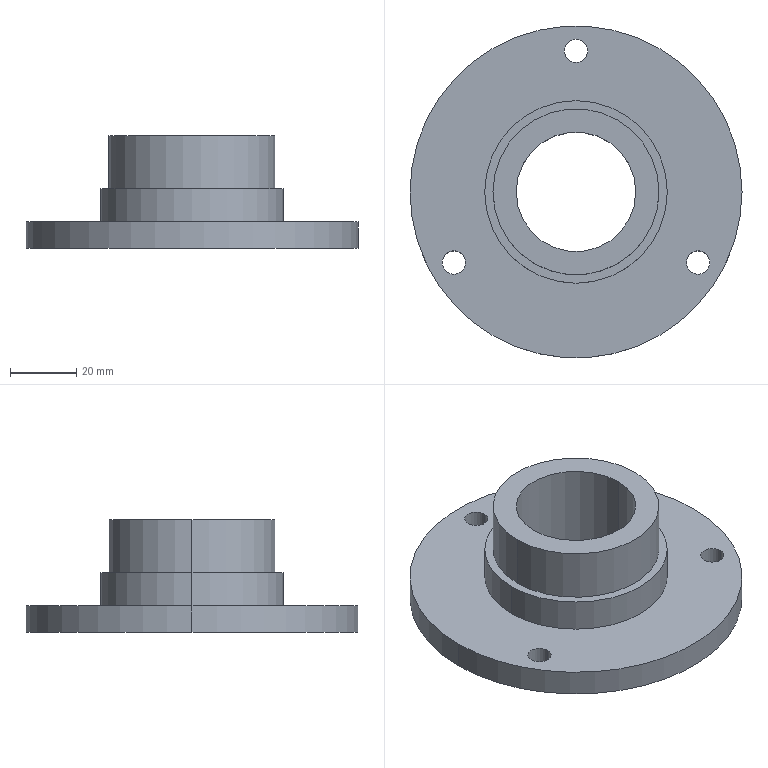Part | SolidWorks | features ICE 2, Extrusion 1 | 1 solid | 18 faces | box 100 x 100 x 34 mm | volume 82475 mm3 | cylinder 14 | plane 4 | commonest cylinder face diameters 7 x6 36 x2 50 x2 55 x2 100 x2
STEP:
#1=CARTESIAN_POINT('',(25.,0.,34.));
#2=VERTEX_POINT('',#1);
#3=CARTESIAN_POINT('',(-25.,0.,34.));
#4=VERTEX_POINT('',#3);
#5=CARTESIAN_POINT('',(0.,0.,34.));
#6=DIRECTION('',(0.,0.,1.));
#7=DIRECTION('',(1.,0.,0.));
#8=AXIS2_PLACEMENT_3D('',#5,#6,#7);
#9=CIRCLE('',#8,25.);
#10=EDGE_CURVE('',#2,#4,#9,.T.);
#11=ORIENTED_EDGE('',*,*,#10,.F.);
#12=CARTESIAN_POINT('',(25.,0.,18.));
#13=VERTEX_POINT('',#12);
#14=CARTESIAN_POINT('',(25.,0.,34.));
#15=DIRECTION('',(0.,0.,-1.));
#16=VECTOR('',#15,1000.);
#17=LINE('',#14,#16);
#18=EDGE_CURVE('',#2,#13,#17,.T.);
#19=ORIENTED_EDGE('',*,*,#18,.T.);
#20=CARTESIAN_POINT('',(-25.,0.,18.));
#21=VERTEX_POINT('',#20);
#22=CARTESIAN_POINT('',(0.,0.,18.));
#23=DIRECTION('',(0.,0.,1.));
#24=DIRECTION('',(1.,0.,0.));
#25=AXIS2_PLACEMENT_3D('',#22,#23,#24);
#26=CIRCLE('',#25,25.);
#27=EDGE_CURVE('',#13,#21,#26,.T.);
#28=ORIENTED_EDGE('',*,*,#27,.T.);
#29=CARTESIAN_POINT('',(-25.,0.,34.));
#30=DIRECTION('',(0.,0.,-1.));
#31=VECTOR('',#30,1000.);
#32=LINE('',#29,#31);
#33=EDGE_CURVE('',#4,#21,#32,.T.);
#34=ORIENTED_EDGE('',*,*,#33,.F.);
#35=EDGE_LOOP('',(#11,#19,#28,#34));
#36=FACE_OUTER_BOUND('',#35,.T.);
#37=CARTESIAN_POINT('',(0.,0.,34.));
#38=DIRECTION('',(0.,0.,-1.));
#39=DIRECTION('',(-1.,0.,0.));
#40=AXIS2_PLACEMENT_3D('',#37,#38,#39);
#41=CYLINDRICAL_SURFACE('',#40,25.);
#42=ADVANCED_FACE('',(#36),#41,.T.);
#43=CARTESIAN_POINT('',(27.5,0.,18.));
#44=VERTEX_POINT('',#43);
#45=CARTESIAN_POINT('',(-27.5,0.,18.));
#46=VERTEX_POINT('',#45);
#47=CARTESIAN_POINT('',(0.,0.,18.));
#48=DIRECTION('',(0.,0.,1.));
#49=DIRECTION('',(1.,0.,0.));
#50=AXIS2_PLACEMENT_3D('',#47,#48,#49);
#51=CIRCLE('',#50,27.5);
#52=EDGE_CURVE('',#44,#46,#51,.T.);
#53=ORIENTED_EDGE('',*,*,#52,.F.);
#54=CARTESIAN_POINT('',(27.5,0.,8.));
#55=VERTEX_POINT('',#54);
#56=CARTESIAN_POINT('',(27.5,0.,18.));
#57=DIRECTION('',(0.,0.,-1.));
#58=VECTOR('',#57,1000.);
#59=LINE('',#56,#58);
#60=EDGE_CURVE('',#44,#55,#59,.T.);
#61=ORIENTED_EDGE('',*,*,#60,.T.);
#62=CARTESIAN_POINT('',(-27.5,0.,8.));
#63=VERTEX_POINT('',#62);
#64=CARTESIAN_POINT('',(0.,0.,8.));
#65=DIRECTION('',(0.,0.,1.));
#66=DIRECTION('',(1.,0.,0.));
#67=AXIS2_PLACEMENT_3D('',#64,#65,#66);
#68=CIRCLE('',#67,27.5);
#69=EDGE_CURVE('',#55,#63,#68,.T.);
#70=ORIENTED_EDGE('',*,*,#69,.T.);
#71=CARTESIAN_POINT('',(-27.5,0.,18.));
#72=DIRECTION('',(0.,0.,-1.));
#73=VECTOR('',#72,1000.);
#74=LINE('',#71,#73);
#75=EDGE_CURVE('',#46,#63,#74,.T.);
#76=ORIENTED_EDGE('',*,*,#75,.F.);
#77=EDGE_LOOP('',(#53,#61,#70,#76));
#78=FACE_OUTER_BOUND('',#77,.T.);
#79=CARTESIAN_POINT('',(0.,0.,18.));
#80=DIRECTION('',(0.,0.,-1.));
#81=DIRECTION('',(-1.,0.,0.));
#82=AXIS2_PLACEMENT_3D('',#79,#80,#81);
#83=CYLINDRICAL_SURFACE('',#82,27.5);
#84=ADVANCED_FACE('',(#78),#83,.T.);
#85=CARTESIAN_POINT('',(-18.,0.,34.));
#86=VERTEX_POINT('',#85);
#87=CARTESIAN_POINT('',(18.,0.,34.));
#88=VERTEX_POINT('',#87);
#89=CARTESIAN_POINT('',(0.,0.,34.));
#90=DIRECTION('',(0.,0.,1.));
#91=DIRECTION('',(1.,0.,0.));
#92=AXIS2_PLACEMENT_3D('',#89,#90,#91);
#93=CIRCLE('',#92,18.);
#94=EDGE_CURVE('',#86,#88,#93,.T.);
#95=ORIENTED_EDGE('',*,*,#94,.T.);
#96=CARTESIAN_POINT('',(18.,0.,0.));
#97=VERTEX_POINT('',#96);
#98=CARTESIAN_POINT('',(18.,0.,8.));
#99=DIRECTION('',(0.,0.,-1.));
#100=VECTOR('',#99,1000.);
#101=LINE('',#98,#100);
#102=EDGE_CURVE('',#88,#97,#101,.T.);
#103=ORIENTED_EDGE('',*,*,#102,.T.);
#104=CARTESIAN_POINT('',(-18.,0.,0.));
#105=VERTEX_POINT('',#104);
#106=CARTESIAN_POINT('',(0.,0.,0.));
#107=DIRECTION('',(0.,0.,1.));
#108=DIRECTION('',(1.,0.,0.));
#109=AXIS2_PLACEMENT_3D('',#106,#107,#108);
#110=CIRCLE('',#109,18.);
#111=EDGE_CURVE('',#105,#97,#110,.T.);
#112=ORIENTED_EDGE('',*,*,#111,.F.);
#113=CARTESIAN_POINT('',(-18.,0.,8.));
#114=DIRECTION('',(0.,0.,-1.));
#115=VECTOR('',#114,1000.);
#116=LINE('',#113,#115);
#117=EDGE_CURVE('',#86,#105,#116,.T.);
#118=ORIENTED_EDGE('',*,*,#117,.F.);
#119=EDGE_LOOP('',(#95,#103,#112,#118));
#120=FACE_OUTER_BOUND('',#119,.T.);
#121=CARTESIAN_POINT('',(0.,0.,8.));
#122=DIRECTION('',(0.,0.,-1.));
#123=DIRECTION('',(-1.,0.,0.));
#124=AXIS2_PLACEMENT_3D('',#121,#122,#123);
#125=CYLINDRICAL_SURFACE('',#124,18.);
#126=ADVANCED_FACE('',(#120),#125,.F.);
#127=CARTESIAN_POINT('',(33.306,-21.25,8.));
#128=VERTEX_POINT('',#127);
#129=CARTESIAN_POINT('',(40.306,-21.25,8.));
#130=VERTEX_POINT('',#129);
#131=CARTESIAN_POINT('',(36.806,-21.25,8.));
#132=DIRECTION('',(0.,0.,1.));
#133=DIRECTION('',(1.,0.,0.));
#134=AXIS2_PLACEMENT_3D('',#131,#132,#133);
#135=CIRCLE('',#134,3.5);
#136=EDGE_CURVE('',#128,#130,#135,.T.);
#137=ORIENTED_EDGE('',*,*,#136,.T.);
#138=CARTESIAN_POINT('',(40.306,-21.25,0.));
#139=VERTEX_POINT('',#138);
#140=CARTESIAN_POINT('',(40.306,-21.25,8.));
#141=DIRECTION('',(0.,0.,-1.));
#142=VECTOR('',#141,1000.);
#143=LINE('',#140,#142);
#144=EDGE_CURVE('',#130,#139,#143,.T.);
#145=ORIENTED_EDGE('',*,*,#144,.T.);
#146=CARTESIAN_POINT('',(33.306,-21.25,0.));
#147=VERTEX_POINT('',#146);
#148=CARTESIAN_POINT('',(36.806,-21.25,0.));
#149=DIRECTION('',(0.,0.,1.));
#150=DIRECTION('',(1.,0.,0.));
#151=AXIS2_PLACEMENT_3D('',#148,#149,#150);
#152=CIRCLE('',#151,3.5);
#153=EDGE_CURVE('',#147,#139,#152,.T.);
#154=ORIENTED_EDGE('',*,*,#153,.F.);
#155=CARTESIAN_POINT('',(33.306,-21.25,8.));
#156=DIRECTION('',(0.,0.,-1.));
#157=VECTOR('',#156,1000.);
#158=LINE('',#155,#157);
#159=EDGE_CURVE('',#128,#147,#158,.T.);
#160=ORIENTED_EDGE('',*,*,#159,.F.);
#161=EDGE_LOOP('',(#137,#145,#154,#160));
#162=FACE_OUTER_BOUND('',#161,.T.);
#163=CARTESIAN_POINT('',(36.806,-21.25,8.));
#164=DIRECTION('',(0.,0.,-1.));
#165=DIRECTION('',(-1.,0.,0.));
#166=AXIS2_PLACEMENT_3D('',#163,#164,#165);
#167=CYLINDRICAL_SURFACE('',#166,3.5);
#168=ADVANCED_FACE('',(#162),#167,.F.);
#169=CARTESIAN_POINT('',(-40.306,-21.25,8.));
#170=VERTEX_POINT('',#169);
#171=CARTESIAN_POINT('',(-33.306,-21.25,8.));
#172=VERTEX_POINT('',#171);
#173=CARTESIAN_POINT('',(-36.806,-21.25,8.));
#174=DIRECTION('',(0.,0.,1.));
#175=DIRECTION('',(1.,0.,0.));
#176=AXIS2_PLACEMENT_3D('',#173,#174,#175);
#177=CIRCLE('',#176,3.5);
#178=EDGE_CURVE('',#170,#172,#177,.T.);
#179=ORIENTED_EDGE('',*,*,#178,.T.);
#180=CARTESIAN_POINT('',(-33.306,-21.25,0.));
#181=VERTEX_POINT('',#180);
#182=CARTESIAN_POINT('',(-33.306,-21.25,8.));
#183=DIRECTION('',(0.,0.,-1.));
#184=VECTOR('',#183,1000.);
#185=LINE('',#182,#184);
#186=EDGE_CURVE('',#172,#181,#185,.T.);
#187=ORIENTED_EDGE('',*,*,#186,.T.);
#188=CARTESIAN_POINT('',(-40.306,-21.25,0.));
#189=VERTEX_POINT('',#188);
#190=CARTESIAN_POINT('',(-36.806,-21.25,0.));
#191=DIRECTION('',(0.,0.,1.));
#192=DIRECTION('',(1.,0.,0.));
#193=AXIS2_PLACEMENT_3D('',#190,#191,#192);
#194=CIRCLE('',#193,3.5);
#195=EDGE_CURVE('',#189,#181,#194,.T.);
#196=ORIENTED_EDGE('',*,*,#195,.F.);
#197=CARTESIAN_POINT('',(-40.306,-21.25,8.));
#198=DIRECTION('',(0.,0.,-1.));
#199=VECTOR('',#198,1000.);
#200=LINE('',#197,#199);
#201=EDGE_CURVE('',#170,#189,#200,.T.);
#202=ORIENTED_EDGE('',*,*,#201,.F.);
#203=EDGE_LOOP('',(#179,#187,#196,#202));
#204=FACE_OUTER_BOUND('',#203,.T.);
#205=CARTESIAN_POINT('',(-36.806,-21.25,8.));
#206=DIRECTION('',(0.,0.,-1.));
#207=DIRECTION('',(-1.,0.,0.));
#208=AXIS2_PLACEMENT_3D('',#205,#206,#207);
#209=CYLINDRICAL_SURFACE('',#208,3.5);
#210=ADVANCED_FACE('',(#204),#209,.F.);
#211=CARTESIAN_POINT('',(-3.5,42.5,8.));
#212=VERTEX_POINT('',#211);
#213=CARTESIAN_POINT('',(3.5,42.5,8.));
#214=VERTEX_POINT('',#213);
#215=CARTESIAN_POINT('',(0.,42.5,8.));
#216=DIRECTION('',(0.,0.,1.));
#217=DIRECTION('',(1.,0.,0.));
#218=AXIS2_PLACEMENT_3D('',#215,#216,#217);
#219=CIRCLE('',#218,3.5);
#220=EDGE_CURVE('',#212,#214,#219,.T.);
#221=ORIENTED_EDGE('',*,*,#220,.T.);
#222=CARTESIAN_POINT('',(3.5,42.5,0.));
#223=VERTEX_POINT('',#222);
#224=CARTESIAN_POINT('',(3.5,42.5,8.));
#225=DIRECTION('',(0.,0.,-1.));
#226=VECTOR('',#225,1000.);
#227=LINE('',#224,#226);
#228=EDGE_CURVE('',#214,#223,#227,.T.);
#229=ORIENTED_EDGE('',*,*,#228,.T.);
#230=CARTESIAN_POINT('',(-3.5,42.5,0.));
#231=VERTEX_POINT('',#230);
#232=CARTESIAN_POINT('',(0.,42.5,0.));
#233=DIRECTION('',(0.,0.,1.));
#234=DIRECTION('',(1.,0.,0.));
#235=AXIS2_PLACEMENT_3D('',#232,#233,#234);
#236=CIRCLE('',#235,3.5);
#237=EDGE_CURVE('',#231,#223,#236,.T.);
#238=ORIENTED_EDGE('',*,*,#237,.F.);
#239=CARTESIAN_POINT('',(-3.5,42.5,8.));
#240=DIRECTION('',(0.,0.,-1.));
#241=VECTOR('',#240,1000.);
#242=LINE('',#239,#241);
#243=EDGE_CURVE('',#212,#231,#242,.T.);
#244=ORIENTED_EDGE('',*,*,#243,.F.);
#245=EDGE_LOOP('',(#221,#229,#238,#244));
#246=FACE_OUTER_BOUND('',#245,.T.);
#247=CARTESIAN_POINT('',(0.,42.5,8.));
#248=DIRECTION('',(0.,0.,-1.));
#249=DIRECTION('',(-1.,0.,0.));
#250=AXIS2_PLACEMENT_3D('',#247,#248,#249);
#251=CYLINDRICAL_SURFACE('',#250,3.5);
#252=ADVANCED_FACE('',(#246),#251,.F.);
#253=CARTESIAN_POINT('',(50.,0.,8.));
#254=VERTEX_POINT('',#253);
#255=CARTESIAN_POINT('',(-50.,0.,8.));
#256=VERTEX_POINT('',#255);
#257=CARTESIAN_POINT('',(0.,0.,8.));
#258=DIRECTION('',(0.,0.,1.));
#259=DIRECTION('',(1.,0.,0.));
#260=AXIS2_PLACEMENT_3D('',#257,#258,#259);
#261=CIRCLE('',#260,50.);
#262=EDGE_CURVE('',#254,#256,#261,.T.);
#263=ORIENTED_EDGE('',*,*,#262,.F.);
#264=CARTESIAN_POINT('',(50.,0.,0.));
#265=VERTEX_POINT('',#264);
#266=CARTESIAN_POINT('',(50.,0.,8.));
#267=DIRECTION('',(0.,0.,-1.));
#268=VECTOR('',#267,1000.);
#269=LINE('',#266,#268);
#270=EDGE_CURVE('',#254,#265,#269,.T.);
#271=ORIENTED_EDGE('',*,*,#270,.T.);
#272=CARTESIAN_POINT('',(-50.,0.,0.));
#273=VERTEX_POINT('',#272);
#274=CARTESIAN_POINT('',(0.,0.,0.));
#275=DIRECTION('',(0.,0.,1.));
#276=DIRECTION('',(1.,0.,0.));
#277=AXIS2_PLACEMENT_3D('',#274,#275,#276);
#278=CIRCLE('',#277,50.);
#279=EDGE_CURVE('',#265,#273,#278,.T.);
#280=ORIENTED_EDGE('',*,*,#279,.T.);
#281=CARTESIAN_POINT('',(-50.,0.,8.));
#282=DIRECTION('',(0.,0.,-1.));
#283=VECTOR('',#282,1000.);
#284=LINE('',#281,#283);
#285=EDGE_CURVE('',#256,#273,#284,.T.);
#286=ORIENTED_EDGE('',*,*,#285,.F.);
#287=EDGE_LOOP('',(#263,#271,#280,#286));
#288=FACE_OUTER_BOUND('',#287,.T.);
#289=CARTESIAN_POINT('',(0.,0.,8.));
#290=DIRECTION('',(0.,0.,-1.));
#291=DIRECTION('',(-1.,0.,0.));
#292=AXIS2_PLACEMENT_3D('',#289,#290,#291);
#293=CYLINDRICAL_SURFACE('',#292,50.);
#294=ADVANCED_FACE('',(#288),#293,.T.);
#295=ORIENTED_EDGE('',*,*,#178,.F.);
#296=CARTESIAN_POINT('',(-36.806,-21.25,8.));
#297=DIRECTION('',(0.,0.,1.));
#298=DIRECTION('',(1.,0.,0.));
#299=AXIS2_PLACEMENT_3D('',#296,#297,#298);
#300=CIRCLE('',#299,3.5);
#301=EDGE_CURVE('',#172,#170,#300,.T.);
#302=ORIENTED_EDGE('',*,*,#301,.F.);
#303=EDGE_LOOP('',(#295,#302));
#304=FACE_BOUND('',#303,.T.);
#305=CARTESIAN_POINT('',(0.,0.,8.));
#306=DIRECTION('',(0.,0.,1.));
#307=DIRECTION('',(1.,0.,0.));
#308=AXIS2_PLACEMENT_3D('',#305,#306,#307);
#309=CIRCLE('',#308,50.);
#310=EDGE_CURVE('',#256,#254,#309,.T.);
#311=ORIENTED_EDGE('',*,*,#310,.T.);
#312=ORIENTED_EDGE('',*,*,#262,.T.);
#313=EDGE_LOOP('',(#311,#312));
#314=FACE_OUTER_BOUND('',#313,.T.);
#315=ORIENTED_EDGE('',*,*,#220,.F.);
#316=CARTESIAN_POINT('',(0.,42.5,8.));
#317=DIRECTION('',(0.,0.,1.));
#318=DIRECTION('',(1.,0.,0.));
#319=AXIS2_PLACEMENT_3D('',#316,#317,#318);
#320=CIRCLE('',#319,3.5);
#321=EDGE_CURVE('',#214,#212,#320,.T.);
#322=ORIENTED_EDGE('',*,*,#321,.F.);
#323=EDGE_LOOP('',(#315,#322));
#324=FACE_BOUND('',#323,.T.);
#325=ORIENTED_EDGE('',*,*,#136,.F.);
#326=CARTESIAN_POINT('',(36.806,-21.25,8.));
#327=DIRECTION('',(0.,0.,1.));
#328=DIRECTION('',(1.,0.,0.));
#329=AXIS2_PLACEMENT_3D('',#326,#327,#328);
#330=CIRCLE('',#329,3.5);
#331=EDGE_CURVE('',#130,#128,#330,.T.);
#332=ORIENTED_EDGE('',*,*,#331,.F.);
#333=EDGE_LOOP('',(#325,#332));
#334=FACE_BOUND('',#333,.T.);
#335=CARTESIAN_POINT('',(0.,0.,8.));
#336=DIRECTION('',(0.,0.,1.));
#337=DIRECTION('',(1.,0.,0.));
#338=AXIS2_PLACEMENT_3D('',#335,#336,#337);
#339=CIRCLE('',#338,27.5);
#340=EDGE_CURVE('',#63,#55,#339,.T.);
#341=ORIENTED_EDGE('',*,*,#340,.F.);
#342=ORIENTED_EDGE('',*,*,#69,.F.);
#343=EDGE_LOOP('',(#341,#342));
#344=FACE_BOUND('',#343,.T.);
#345=CARTESIAN_POINT('',(0.,0.,8.));
#346=DIRECTION('',(0.,0.,1.));
#347=DIRECTION('',(1.,0.,0.));
#348=AXIS2_PLACEMENT_3D('',#345,#346,#347);
#349=PLANE('',#348);
#350=ADVANCED_FACE('',(#304,#314,#324,#334,#344),#349,.T.);
#351=CARTESIAN_POINT('',(0.,0.,0.));
#352=DIRECTION('',(0.,0.,1.));
#353=DIRECTION('',(1.,0.,0.));
#354=AXIS2_PLACEMENT_3D('',#351,#352,#353);
#355=CIRCLE('',#354,50.);
#356=EDGE_CURVE('',#273,#265,#355,.T.);
#357=ORIENTED_EDGE('',*,*,#356,.F.);
#358=ORIENTED_EDGE('',*,*,#279,.F.);
#359=EDGE_LOOP('',(#357,#358));
#360=FACE_OUTER_BOUND('',#359,.T.);
#361=ORIENTED_EDGE('',*,*,#237,.T.);
#362=CARTESIAN_POINT('',(0.,42.5,0.));
#363=DIRECTION('',(0.,0.,1.));
#364=DIRECTION('',(1.,0.,0.));
#365=AXIS2_PLACEMENT_3D('',#362,#363,#364);
#366=CIRCLE('',#365,3.5);
#367=EDGE_CURVE('',#223,#231,#366,.T.);
#368=ORIENTED_EDGE('',*,*,#367,.T.);
#369=EDGE_LOOP('',(#361,#368));
#370=FACE_BOUND('',#369,.T.);
#371=ORIENTED_EDGE('',*,*,#195,.T.);
#372=CARTESIAN_POINT('',(-36.806,-21.25,0.));
#373=DIRECTION('',(0.,0.,1.));
#374=DIRECTION('',(1.,0.,0.));
#375=AXIS2_PLACEMENT_3D('',#372,#373,#374);
#376=CIRCLE('',#375,3.5);
#377=EDGE_CURVE('',#181,#189,#376,.T.);
#378=ORIENTED_EDGE('',*,*,#377,.T.);
#379=EDGE_LOOP('',(#371,#378));
#380=FACE_BOUND('',#379,.T.);
#381=ORIENTED_EDGE('',*,*,#153,.T.);
#382=CARTESIAN_POINT('',(36.806,-21.25,0.));
#383=DIRECTION('',(0.,0.,1.));
#384=DIRECTION('',(1.,0.,0.));
#385=AXIS2_PLACEMENT_3D('',#382,#383,#384);
#386=CIRCLE('',#385,3.5);
#387=EDGE_CURVE('',#139,#147,#386,.T.);
#388=ORIENTED_EDGE('',*,*,#387,.T.);
#389=EDGE_LOOP('',(#381,#388));
#390=FACE_BOUND('',#389,.T.);
#391=ORIENTED_EDGE('',*,*,#111,.T.);
#392=CARTESIAN_POINT('',(0.,0.,0.));
#393=DIRECTION('',(0.,0.,1.));
#394=DIRECTION('',(1.,0.,0.));
#395=AXIS2_PLACEMENT_3D('',#392,#393,#394);
#396=CIRCLE('',#395,18.);
#397=EDGE_CURVE('',#97,#105,#396,.T.);
#398=ORIENTED_EDGE('',*,*,#397,.T.);
#399=EDGE_LOOP('',(#391,#398));
#400=FACE_BOUND('',#399,.T.);
#401=CARTESIAN_POINT('',(0.,0.,0.));
#402=DIRECTION('',(0.,0.,1.));
#403=DIRECTION('',(1.,0.,0.));
#404=AXIS2_PLACEMENT_3D('',#401,#402,#403);
#405=PLANE('',#404);
#406=ADVANCED_FACE('',(#360,#370,#380,#390,#400),#405,.F.);
#407=ORIENTED_EDGE('',*,*,#270,.F.);
#408=ORIENTED_EDGE('',*,*,#310,.F.);
#409=ORIENTED_EDGE('',*,*,#285,.T.);
#410=ORIENTED_EDGE('',*,*,#356,.T.);
#411=EDGE_LOOP('',(#407,#408,#409,#410));
#412=FACE_OUTER_BOUND('',#411,.T.);
#413=CARTESIAN_POINT('',(0.,0.,8.));
#414=DIRECTION('',(0.,0.,-1.));
#415=DIRECTION('',(-1.,0.,0.));
#416=AXIS2_PLACEMENT_3D('',#413,#414,#415);
#417=CYLINDRICAL_SURFACE('',#416,50.);
#418=ADVANCED_FACE('',(#412),#417,.T.);
#419=ORIENTED_EDGE('',*,*,#228,.F.);
#420=ORIENTED_EDGE('',*,*,#321,.T.);
#421=ORIENTED_EDGE('',*,*,#243,.T.);
#422=ORIENTED_EDGE('',*,*,#367,.F.);
#423=EDGE_LOOP('',(#419,#420,#421,#422));
#424=FACE_OUTER_BOUND('',#423,.T.);
#425=CARTESIAN_POINT('',(0.,42.5,8.));
#426=DIRECTION('',(0.,0.,-1.));
#427=DIRECTION('',(-1.,0.,0.));
#428=AXIS2_PLACEMENT_3D('',#425,#426,#427);
#429=CYLINDRICAL_SURFACE('',#428,3.5);
#430=ADVANCED_FACE('',(#424),#429,.F.);
#431=ORIENTED_EDGE('',*,*,#186,.F.);
#432=ORIENTED_EDGE('',*,*,#301,.T.);
#433=ORIENTED_EDGE('',*,*,#201,.T.);
#434=ORIENTED_EDGE('',*,*,#377,.F.);
#435=EDGE_LOOP('',(#431,#432,#433,#434));
#436=FACE_OUTER_BOUND('',#435,.T.);
#437=CARTESIAN_POINT('',(-36.806,-21.25,8.));
#438=DIRECTION('',(0.,0.,-1.));
#439=DIRECTION('',(-1.,0.,0.));
#440=AXIS2_PLACEMENT_3D('',#437,#438,#439);
#441=CYLINDRICAL_SURFACE('',#440,3.5);
#442=ADVANCED_FACE('',(#436),#441,.F.);
#443=ORIENTED_EDGE('',*,*,#144,.F.);
#444=ORIENTED_EDGE('',*,*,#331,.T.);
#445=ORIENTED_EDGE('',*,*,#159,.T.);
#446=ORIENTED_EDGE('',*,*,#387,.F.);
#447=EDGE_LOOP('',(#443,#444,#445,#446));
#448=FACE_OUTER_BOUND('',#447,.T.);
#449=CARTESIAN_POINT('',(36.806,-21.25,8.));
#450=DIRECTION('',(0.,0.,-1.));
#451=DIRECTION('',(-1.,0.,0.));
#452=AXIS2_PLACEMENT_3D('',#449,#450,#451);
#453=CYLINDRICAL_SURFACE('',#452,3.5);
#454=ADVANCED_FACE('',(#448),#453,.F.);
#455=ORIENTED_EDGE('',*,*,#102,.F.);
#456=CARTESIAN_POINT('',(0.,0.,34.));
#457=DIRECTION('',(0.,0.,1.));
#458=DIRECTION('',(1.,0.,0.));
#459=AXIS2_PLACEMENT_3D('',#456,#457,#458);
#460=CIRCLE('',#459,18.);
#461=EDGE_CURVE('',#88,#86,#460,.T.);
#462=ORIENTED_EDGE('',*,*,#461,.T.);
#463=ORIENTED_EDGE('',*,*,#117,.T.);
#464=ORIENTED_EDGE('',*,*,#397,.F.);
#465=EDGE_LOOP('',(#455,#462,#463,#464));
#466=FACE_OUTER_BOUND('',#465,.T.);
#467=CARTESIAN_POINT('',(0.,0.,8.));
#468=DIRECTION('',(0.,0.,-1.));
#469=DIRECTION('',(-1.,0.,0.));
#470=AXIS2_PLACEMENT_3D('',#467,#468,#469);
#471=CYLINDRICAL_SURFACE('',#470,18.);
#472=ADVANCED_FACE('',(#466),#471,.F.);
#473=CARTESIAN_POINT('',(0.,0.,18.));
#474=DIRECTION('',(0.,0.,1.));
#475=DIRECTION('',(1.,0.,0.));
#476=AXIS2_PLACEMENT_3D('',#473,#474,#475);
#477=CIRCLE('',#476,25.);
#478=EDGE_CURVE('',#21,#13,#477,.T.);
#479=ORIENTED_EDGE('',*,*,#478,.F.);
#480=ORIENTED_EDGE('',*,*,#27,.F.);
#481=EDGE_LOOP('',(#479,#480));
#482=FACE_BOUND('',#481,.T.);
#483=CARTESIAN_POINT('',(0.,0.,18.));
#484=DIRECTION('',(0.,0.,1.));
#485=DIRECTION('',(1.,0.,0.));
#486=AXIS2_PLACEMENT_3D('',#483,#484,#485);
#487=CIRCLE('',#486,27.5);
#488=EDGE_CURVE('',#46,#44,#487,.T.);
#489=ORIENTED_EDGE('',*,*,#488,.T.);
#490=ORIENTED_EDGE('',*,*,#52,.T.);
#491=EDGE_LOOP('',(#489,#490));
#492=FACE_OUTER_BOUND('',#491,.T.);
#493=CARTESIAN_POINT('',(0.,0.,18.));
#494=DIRECTION('',(0.,0.,1.));
#495=DIRECTION('',(1.,0.,0.));
#496=AXIS2_PLACEMENT_3D('',#493,#494,#495);
#497=PLANE('',#496);
#498=ADVANCED_FACE('',(#482,#492),#497,.T.);
#499=ORIENTED_EDGE('',*,*,#60,.F.);
#500=ORIENTED_EDGE('',*,*,#488,.F.);
#501=ORIENTED_EDGE('',*,*,#75,.T.);
#502=ORIENTED_EDGE('',*,*,#340,.T.);
#503=EDGE_LOOP('',(#499,#500,#501,#502));
#504=FACE_OUTER_BOUND('',#503,.T.);
#505=CARTESIAN_POINT('',(0.,0.,18.));
#506=DIRECTION('',(0.,0.,-1.));
#507=DIRECTION('',(-1.,0.,0.));
#508=AXIS2_PLACEMENT_3D('',#505,#506,#507);
#509=CYLINDRICAL_SURFACE('',#508,27.5);
#510=ADVANCED_FACE('',(#504),#509,.T.);
#511=CARTESIAN_POINT('',(0.,0.,34.));
#512=DIRECTION('',(0.,0.,1.));
#513=DIRECTION('',(1.,0.,0.));
#514=AXIS2_PLACEMENT_3D('',#511,#512,#513);
#515=CIRCLE('',#514,25.);
#516=EDGE_CURVE('',#4,#2,#515,.T.);
#517=ORIENTED_EDGE('',*,*,#516,.T.);
#518=ORIENTED_EDGE('',*,*,#10,.T.);
#519=EDGE_LOOP('',(#517,#518));
#520=FACE_OUTER_BOUND('',#519,.T.);
#521=ORIENTED_EDGE('',*,*,#94,.F.);
#522=ORIENTED_EDGE('',*,*,#461,.F.);
#523=EDGE_LOOP('',(#521,#522));
#524=FACE_BOUND('',#523,.T.);
#525=CARTESIAN_POINT('',(0.,0.,34.));
#526=DIRECTION('',(0.,0.,1.));
#527=DIRECTION('',(1.,0.,0.));
#528=AXIS2_PLACEMENT_3D('',#525,#526,#527);
#529=PLANE('',#528);
#530=ADVANCED_FACE('',(#520,#524),#529,.T.);
#531=ORIENTED_EDGE('',*,*,#18,.F.);
#532=ORIENTED_EDGE('',*,*,#516,.F.);
#533=ORIENTED_EDGE('',*,*,#33,.T.);
#534=ORIENTED_EDGE('',*,*,#478,.T.);
#535=EDGE_LOOP('',(#531,#532,#533,#534));
#536=FACE_OUTER_BOUND('',#535,.T.);
#537=CARTESIAN_POINT('',(0.,0.,34.));
#538=DIRECTION('',(0.,0.,-1.));
#539=DIRECTION('',(-1.,0.,0.));
#540=AXIS2_PLACEMENT_3D('',#537,#538,#539);
#541=CYLINDRICAL_SURFACE('',#540,25.);
#542=ADVANCED_FACE('',(#536),#541,.T.);
#543=CLOSED_SHELL('',(#42,#84,#126,#168,#210,#252,#294,#350,#406,#418,#430,#442,#454,#472,#498,#510,#530,#542));
#544=MANIFOLD_SOLID_BREP('',#543);
#545=CARTESIAN_POINT('',(0.,0.,0.));
#546=DIRECTION('',(0.,0.,1.));
#547=DIRECTION('',(1.,0.,0.));
#548=AXIS2_PLACEMENT_3D('',#545,#546,#547);
#549=(LENGTH_UNIT()NAMED_UNIT(*)SI_UNIT(.MILLI.,.METRE.));
#550=UNCERTAINTY_MEASURE_WITH_UNIT(LENGTH_MEASURE(0.00001),#549,'','');
#551=(NAMED_UNIT(*)PLANE_ANGLE_UNIT()SI_UNIT($,.RADIAN.));
#552=(NAMED_UNIT(*)SI_UNIT($,.STERADIAN.)SOLID_ANGLE_UNIT());
#553=(GEOMETRIC_REPRESENTATION_CONTEXT(3)GLOBAL_UNCERTAINTY_ASSIGNED_CONTEXT((#550))GLOBAL_UNIT_ASSIGNED_CONTEXT((#549,#551,#552))REPRESENTATION_CONTEXT('',''));
#554=ADVANCED_BREP_SHAPE_REPRESENTATION('',(#544,#548),#553);